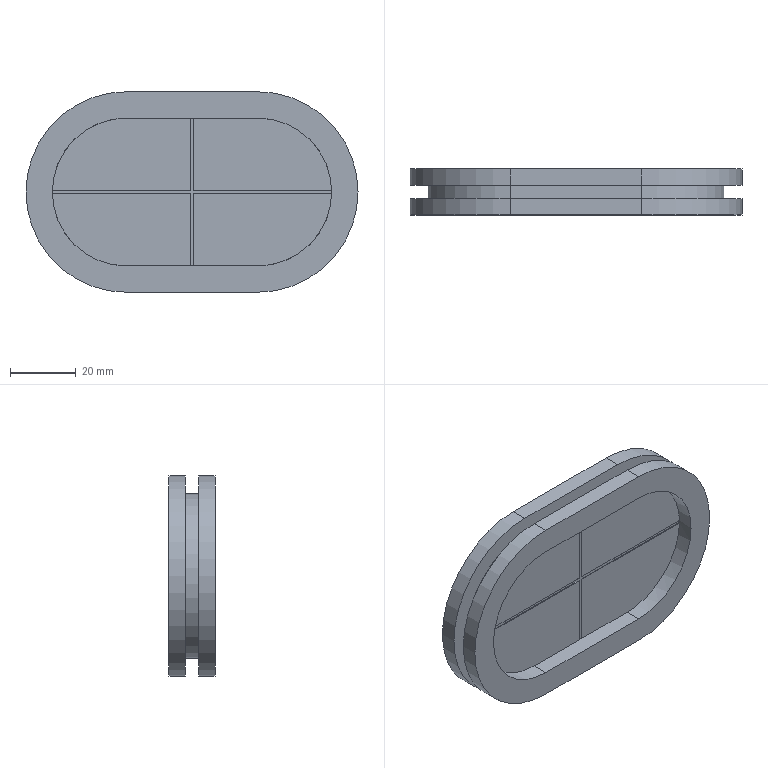Part | SolidWorks | features BaseBody 1 | 1 solid | 54 faces | box 101 x 14 x 61 mm | volume 35523 mm3 | plane 44 | cylinder 10 | commonest cylinder face diameters 45 x4 61 x4 50 x2